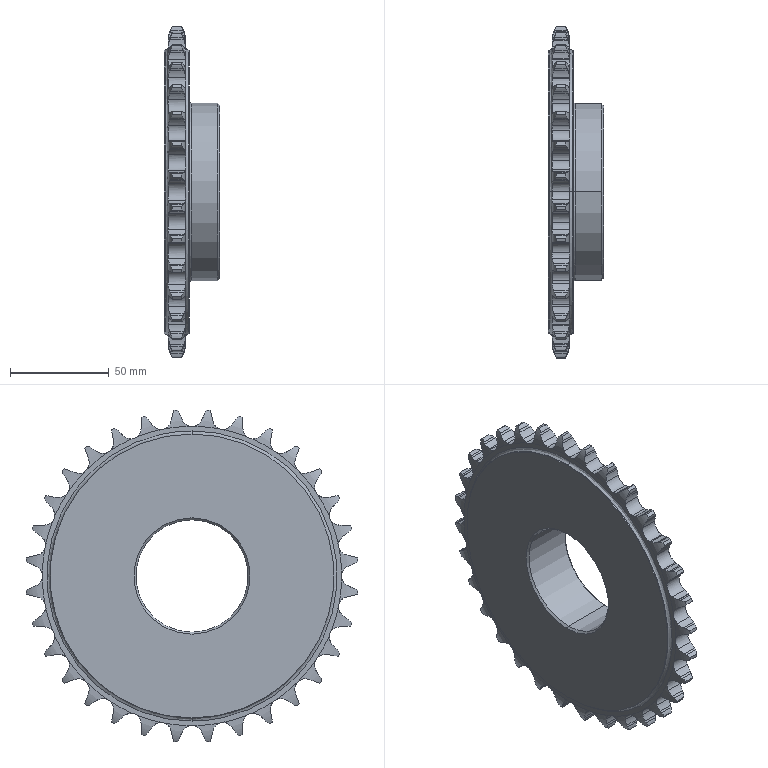Part | STEP file | PN_0021_driven sprocket_05B | 1 solid | 362 faces | box 28 x 168.348 x 168.348 mm | volume 260352 mm3 | cylinder 217 | spline 70 | plane 69 | cone 6 | commonest cylinder face diameters 14.556 x68 26.567 x68 10.311 x41 169 x32 144 x4 57 x2